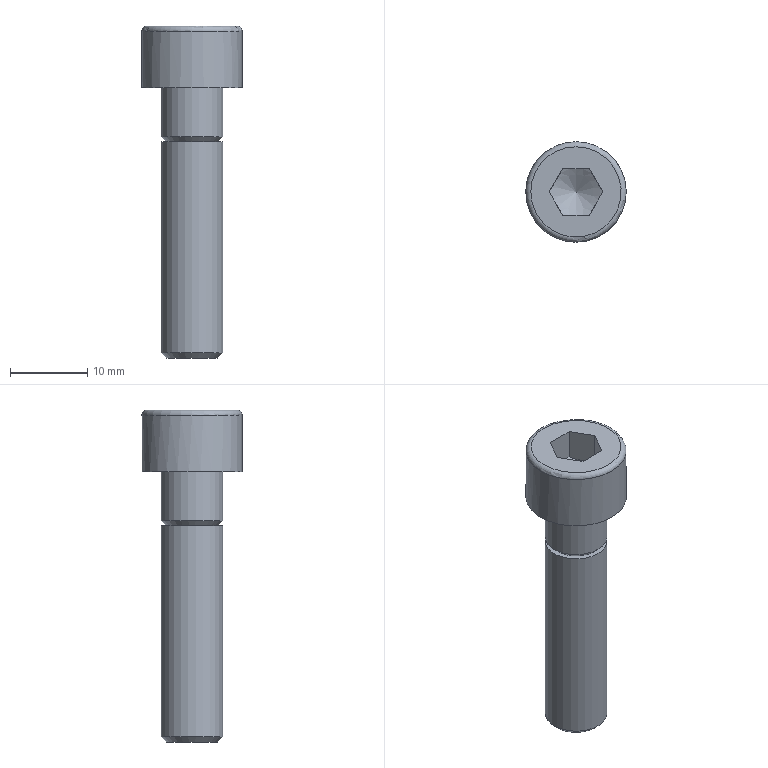Part | STEP file | 1_20 | 1 solid | 17 faces | box 13 x 13 x 43 mm | volume 2658 mm3 | plane 10 | cylinder 3 | cone 3 | torus 1 | commonest cylinder face diameters 8 x2 13 x1